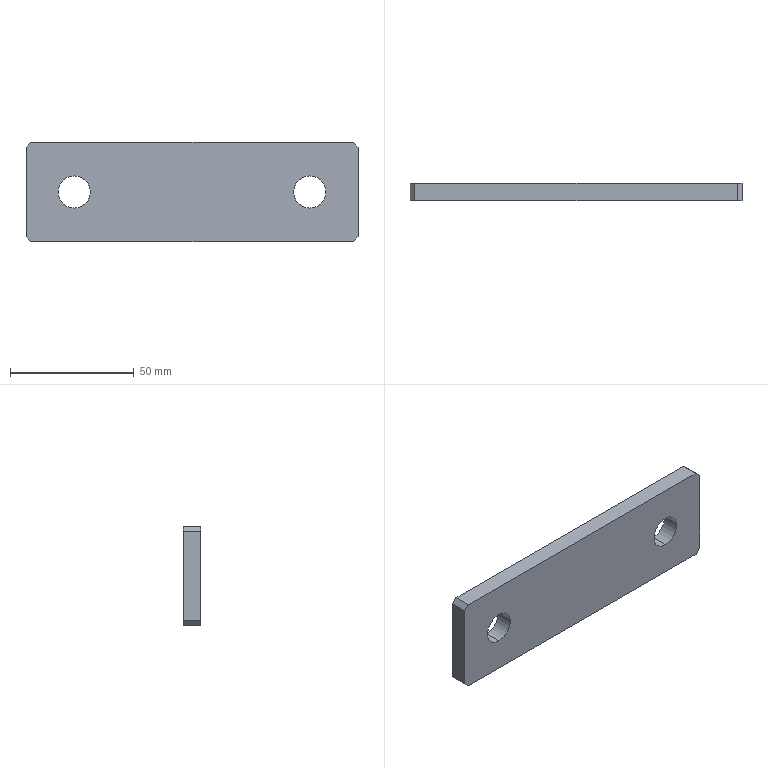Part | STEP file | 1004-2001-0021_1004-2001-0021_1-2 | 1 solid | 14 faces | box 134 x 7 x 40 mm | volume 35606 mm3 | plane 10 | cylinder 4 | commonest cylinder face diameters 13 x4
STEP:
#1=CARTESIAN_POINT('',(-47.5,-3.5,6.5));
#2=VERTEX_POINT('',#1);
#3=CARTESIAN_POINT('',(-47.5,-3.5,-6.5));
#4=VERTEX_POINT('',#3);
#5=CARTESIAN_POINT('',(-47.5,-3.5,0.));
#6=DIRECTION('',(0.,-1.,0.));
#7=DIRECTION('',(0.,0.,1.));
#8=AXIS2_PLACEMENT_3D('',#5,#6,#7);
#9=CIRCLE('',#8,6.5);
#10=EDGE_CURVE('',#2,#4,#9,.T.);
#11=ORIENTED_EDGE('',*,*,#10,.T.);
#12=CARTESIAN_POINT('',(-47.5,3.5,-6.5));
#13=VERTEX_POINT('',#12);
#14=CARTESIAN_POINT('',(-47.5,3.5,-6.5));
#15=DIRECTION('',(0.,1.,0.));
#16=VECTOR('',#15,1000.);
#17=LINE('',#14,#16);
#18=EDGE_CURVE('',#4,#13,#17,.T.);
#19=ORIENTED_EDGE('',*,*,#18,.T.);
#20=CARTESIAN_POINT('',(-47.5,3.5,6.5));
#21=VERTEX_POINT('',#20);
#22=CARTESIAN_POINT('',(-47.5,3.5,0.));
#23=DIRECTION('',(0.,-1.,0.));
#24=DIRECTION('',(0.,0.,1.));
#25=AXIS2_PLACEMENT_3D('',#22,#23,#24);
#26=CIRCLE('',#25,6.5);
#27=EDGE_CURVE('',#21,#13,#26,.T.);
#28=ORIENTED_EDGE('',*,*,#27,.F.);
#29=CARTESIAN_POINT('',(-47.5,3.5,6.5));
#30=DIRECTION('',(0.,1.,0.));
#31=VECTOR('',#30,1000.);
#32=LINE('',#29,#31);
#33=EDGE_CURVE('',#2,#21,#32,.T.);
#34=ORIENTED_EDGE('',*,*,#33,.F.);
#35=EDGE_LOOP('',(#11,#19,#28,#34));
#36=FACE_OUTER_BOUND('',#35,.T.);
#37=CARTESIAN_POINT('',(-47.5,3.5,0.));
#38=DIRECTION('',(0.,1.,0.));
#39=DIRECTION('',(0.,0.,1.));
#40=AXIS2_PLACEMENT_3D('',#37,#38,#39);
#41=CYLINDRICAL_SURFACE('',#40,6.5);
#42=ADVANCED_FACE('',(#36),#41,.F.);
#43=CARTESIAN_POINT('',(47.5,-3.5,6.5));
#44=VERTEX_POINT('',#43);
#45=CARTESIAN_POINT('',(47.5,-3.5,-6.5));
#46=VERTEX_POINT('',#45);
#47=CARTESIAN_POINT('',(47.5,-3.5,0.));
#48=DIRECTION('',(0.,-1.,0.));
#49=DIRECTION('',(0.,0.,1.));
#50=AXIS2_PLACEMENT_3D('',#47,#48,#49);
#51=CIRCLE('',#50,6.5);
#52=EDGE_CURVE('',#44,#46,#51,.T.);
#53=ORIENTED_EDGE('',*,*,#52,.T.);
#54=CARTESIAN_POINT('',(47.5,3.5,-6.5));
#55=VERTEX_POINT('',#54);
#56=CARTESIAN_POINT('',(47.5,3.5,-6.5));
#57=DIRECTION('',(0.,1.,0.));
#58=VECTOR('',#57,1000.);
#59=LINE('',#56,#58);
#60=EDGE_CURVE('',#46,#55,#59,.T.);
#61=ORIENTED_EDGE('',*,*,#60,.T.);
#62=CARTESIAN_POINT('',(47.5,3.5,6.5));
#63=VERTEX_POINT('',#62);
#64=CARTESIAN_POINT('',(47.5,3.5,0.));
#65=DIRECTION('',(0.,-1.,0.));
#66=DIRECTION('',(0.,0.,1.));
#67=AXIS2_PLACEMENT_3D('',#64,#65,#66);
#68=CIRCLE('',#67,6.5);
#69=EDGE_CURVE('',#63,#55,#68,.T.);
#70=ORIENTED_EDGE('',*,*,#69,.F.);
#71=CARTESIAN_POINT('',(47.5,3.5,6.5));
#72=DIRECTION('',(0.,1.,0.));
#73=VECTOR('',#72,1000.);
#74=LINE('',#71,#73);
#75=EDGE_CURVE('',#44,#63,#74,.T.);
#76=ORIENTED_EDGE('',*,*,#75,.F.);
#77=EDGE_LOOP('',(#53,#61,#70,#76));
#78=FACE_OUTER_BOUND('',#77,.T.);
#79=CARTESIAN_POINT('',(47.5,3.5,0.));
#80=DIRECTION('',(0.,1.,0.));
#81=DIRECTION('',(0.,0.,1.));
#82=AXIS2_PLACEMENT_3D('',#79,#80,#81);
#83=CYLINDRICAL_SURFACE('',#82,6.5);
#84=ADVANCED_FACE('',(#78),#83,.F.);
#85=ORIENTED_EDGE('',*,*,#10,.F.);
#86=CARTESIAN_POINT('',(-47.5,-3.5,0.));
#87=DIRECTION('',(0.,-1.,0.));
#88=DIRECTION('',(0.,0.,1.));
#89=AXIS2_PLACEMENT_3D('',#86,#87,#88);
#90=CIRCLE('',#89,6.5);
#91=EDGE_CURVE('',#4,#2,#90,.T.);
#92=ORIENTED_EDGE('',*,*,#91,.F.);
#93=EDGE_LOOP('',(#85,#92));
#94=FACE_BOUND('',#93,.T.);
#95=ORIENTED_EDGE('',*,*,#52,.F.);
#96=CARTESIAN_POINT('',(47.5,-3.5,0.));
#97=DIRECTION('',(0.,-1.,0.));
#98=DIRECTION('',(0.,0.,1.));
#99=AXIS2_PLACEMENT_3D('',#96,#97,#98);
#100=CIRCLE('',#99,6.5);
#101=EDGE_CURVE('',#46,#44,#100,.T.);
#102=ORIENTED_EDGE('',*,*,#101,.F.);
#103=EDGE_LOOP('',(#95,#102));
#104=FACE_BOUND('',#103,.T.);
#105=CARTESIAN_POINT('',(65.,-3.5,-20.));
#106=VERTEX_POINT('',#105);
#107=CARTESIAN_POINT('',(-65.,-3.5,-20.));
#108=VERTEX_POINT('',#107);
#109=CARTESIAN_POINT('',(67.,-3.5,-20.));
#110=DIRECTION('',(-1.,0.,0.));
#111=VECTOR('',#110,1000.);
#112=LINE('',#109,#111);
#113=EDGE_CURVE('',#106,#108,#112,.T.);
#114=ORIENTED_EDGE('',*,*,#113,.F.);
#115=CARTESIAN_POINT('',(67.,-3.5,-18.));
#116=VERTEX_POINT('',#115);
#117=CARTESIAN_POINT('',(67.,-3.5,-18.));
#118=DIRECTION('',(-0.7071,0.,-0.7071));
#119=VECTOR('',#118,1000.);
#120=LINE('',#117,#119);
#121=EDGE_CURVE('',#116,#106,#120,.T.);
#122=ORIENTED_EDGE('',*,*,#121,.F.);
#123=CARTESIAN_POINT('',(67.,-3.5,18.));
#124=VERTEX_POINT('',#123);
#125=CARTESIAN_POINT('',(67.,-3.5,-20.));
#126=DIRECTION('',(0.,0.,-1.));
#127=VECTOR('',#126,1000.);
#128=LINE('',#125,#127);
#129=EDGE_CURVE('',#124,#116,#128,.T.);
#130=ORIENTED_EDGE('',*,*,#129,.F.);
#131=CARTESIAN_POINT('',(65.,-3.5,20.));
#132=VERTEX_POINT('',#131);
#133=CARTESIAN_POINT('',(65.,-3.5,20.));
#134=DIRECTION('',(0.7071,0.,-0.7071));
#135=VECTOR('',#134,1000.);
#136=LINE('',#133,#135);
#137=EDGE_CURVE('',#132,#124,#136,.T.);
#138=ORIENTED_EDGE('',*,*,#137,.F.);
#139=CARTESIAN_POINT('',(-65.,-3.5,20.));
#140=VERTEX_POINT('',#139);
#141=CARTESIAN_POINT('',(67.,-3.5,20.));
#142=DIRECTION('',(1.,0.,0.));
#143=VECTOR('',#142,1000.);
#144=LINE('',#141,#143);
#145=EDGE_CURVE('',#140,#132,#144,.T.);
#146=ORIENTED_EDGE('',*,*,#145,.F.);
#147=CARTESIAN_POINT('',(-67.,-3.5,18.));
#148=VERTEX_POINT('',#147);
#149=CARTESIAN_POINT('',(-67.,-3.5,18.));
#150=DIRECTION('',(0.7071,0.,0.7071));
#151=VECTOR('',#150,1000.);
#152=LINE('',#149,#151);
#153=EDGE_CURVE('',#148,#140,#152,.T.);
#154=ORIENTED_EDGE('',*,*,#153,.F.);
#155=CARTESIAN_POINT('',(-67.,-3.5,-18.));
#156=VERTEX_POINT('',#155);
#157=CARTESIAN_POINT('',(-67.,-3.5,-20.));
#158=DIRECTION('',(0.,0.,1.));
#159=VECTOR('',#158,1000.);
#160=LINE('',#157,#159);
#161=EDGE_CURVE('',#156,#148,#160,.T.);
#162=ORIENTED_EDGE('',*,*,#161,.F.);
#163=CARTESIAN_POINT('',(-65.,-3.5,-20.));
#164=DIRECTION('',(-0.7071,0.,0.7071));
#165=VECTOR('',#164,1000.);
#166=LINE('',#163,#165);
#167=EDGE_CURVE('',#108,#156,#166,.T.);
#168=ORIENTED_EDGE('',*,*,#167,.F.);
#169=EDGE_LOOP('',(#114,#122,#130,#138,#146,#154,#162,#168));
#170=FACE_OUTER_BOUND('',#169,.T.);
#171=CARTESIAN_POINT('',(67.,-3.5,-20.));
#172=DIRECTION('',(0.,1.,0.));
#173=DIRECTION('',(0.,0.,1.));
#174=AXIS2_PLACEMENT_3D('',#171,#172,#173);
#175=PLANE('',#174);
#176=ADVANCED_FACE('',(#94,#104,#170),#175,.F.);
#177=ORIENTED_EDGE('',*,*,#18,.F.);
#178=ORIENTED_EDGE('',*,*,#91,.T.);
#179=ORIENTED_EDGE('',*,*,#33,.T.);
#180=CARTESIAN_POINT('',(-47.5,3.5,0.));
#181=DIRECTION('',(0.,-1.,0.));
#182=DIRECTION('',(0.,0.,1.));
#183=AXIS2_PLACEMENT_3D('',#180,#181,#182);
#184=CIRCLE('',#183,6.5);
#185=EDGE_CURVE('',#13,#21,#184,.T.);
#186=ORIENTED_EDGE('',*,*,#185,.F.);
#187=EDGE_LOOP('',(#177,#178,#179,#186));
#188=FACE_OUTER_BOUND('',#187,.T.);
#189=CARTESIAN_POINT('',(-47.5,3.5,0.));
#190=DIRECTION('',(0.,1.,0.));
#191=DIRECTION('',(0.,0.,1.));
#192=AXIS2_PLACEMENT_3D('',#189,#190,#191);
#193=CYLINDRICAL_SURFACE('',#192,6.5);
#194=ADVANCED_FACE('',(#188),#193,.F.);
#195=ORIENTED_EDGE('',*,*,#60,.F.);
#196=ORIENTED_EDGE('',*,*,#101,.T.);
#197=ORIENTED_EDGE('',*,*,#75,.T.);
#198=CARTESIAN_POINT('',(47.5,3.5,0.));
#199=DIRECTION('',(0.,-1.,0.));
#200=DIRECTION('',(0.,0.,1.));
#201=AXIS2_PLACEMENT_3D('',#198,#199,#200);
#202=CIRCLE('',#201,6.5);
#203=EDGE_CURVE('',#55,#63,#202,.T.);
#204=ORIENTED_EDGE('',*,*,#203,.F.);
#205=EDGE_LOOP('',(#195,#196,#197,#204));
#206=FACE_OUTER_BOUND('',#205,.T.);
#207=CARTESIAN_POINT('',(47.5,3.5,0.));
#208=DIRECTION('',(0.,1.,0.));
#209=DIRECTION('',(0.,0.,1.));
#210=AXIS2_PLACEMENT_3D('',#207,#208,#209);
#211=CYLINDRICAL_SURFACE('',#210,6.5);
#212=ADVANCED_FACE('',(#206),#211,.F.);
#213=CARTESIAN_POINT('',(-65.,3.5,-20.));
#214=VERTEX_POINT('',#213);
#215=CARTESIAN_POINT('',(-67.,3.5,-18.));
#216=VERTEX_POINT('',#215);
#217=CARTESIAN_POINT('',(-65.,3.5,-20.));
#218=DIRECTION('',(-0.7071,0.,0.7071));
#219=VECTOR('',#218,1000.);
#220=LINE('',#217,#219);
#221=EDGE_CURVE('',#214,#216,#220,.T.);
#222=ORIENTED_EDGE('',*,*,#221,.F.);
#223=CARTESIAN_POINT('',(-65.,-3.5,-20.));
#224=DIRECTION('',(0.,1.,0.));
#225=VECTOR('',#224,1000.);
#226=LINE('',#223,#225);
#227=EDGE_CURVE('',#108,#214,#226,.T.);
#228=ORIENTED_EDGE('',*,*,#227,.F.);
#229=ORIENTED_EDGE('',*,*,#167,.T.);
#230=CARTESIAN_POINT('',(-67.,-3.5,-18.));
#231=DIRECTION('',(0.,-1.,0.));
#232=VECTOR('',#231,1000.);
#233=LINE('',#230,#232);
#234=EDGE_CURVE('',#216,#156,#233,.T.);
#235=ORIENTED_EDGE('',*,*,#234,.F.);
#236=EDGE_LOOP('',(#222,#228,#229,#235));
#237=FACE_OUTER_BOUND('',#236,.T.);
#238=CARTESIAN_POINT('',(-65.,-3.5,-20.));
#239=DIRECTION('',(0.7071,0.,0.7071));
#240=DIRECTION('',(0.7071,0.,-0.7071));
#241=AXIS2_PLACEMENT_3D('',#238,#239,#240);
#242=PLANE('',#241);
#243=ADVANCED_FACE('',(#237),#242,.F.);
#244=CARTESIAN_POINT('',(65.,3.5,-20.));
#245=VERTEX_POINT('',#244);
#246=CARTESIAN_POINT('',(67.,3.5,-20.));
#247=DIRECTION('',(-1.,0.,0.));
#248=VECTOR('',#247,1000.);
#249=LINE('',#246,#248);
#250=EDGE_CURVE('',#245,#214,#249,.T.);
#251=ORIENTED_EDGE('',*,*,#250,.F.);
#252=CARTESIAN_POINT('',(65.,-3.5,-20.));
#253=DIRECTION('',(0.,1.,0.));
#254=VECTOR('',#253,1000.);
#255=LINE('',#252,#254);
#256=EDGE_CURVE('',#106,#245,#255,.T.);
#257=ORIENTED_EDGE('',*,*,#256,.F.);
#258=ORIENTED_EDGE('',*,*,#113,.T.);
#259=ORIENTED_EDGE('',*,*,#227,.T.);
#260=EDGE_LOOP('',(#251,#257,#258,#259));
#261=FACE_OUTER_BOUND('',#260,.T.);
#262=CARTESIAN_POINT('',(67.,-3.5,-20.));
#263=DIRECTION('',(0.,0.,1.));
#264=DIRECTION('',(1.,0.,0.));
#265=AXIS2_PLACEMENT_3D('',#262,#263,#264);
#266=PLANE('',#265);
#267=ADVANCED_FACE('',(#261),#266,.F.);
#268=CARTESIAN_POINT('',(67.,3.5,-18.));
#269=VERTEX_POINT('',#268);
#270=CARTESIAN_POINT('',(67.,3.5,-18.));
#271=DIRECTION('',(0.,-1.,0.));
#272=VECTOR('',#271,1000.);
#273=LINE('',#270,#272);
#274=EDGE_CURVE('',#269,#116,#273,.T.);
#275=ORIENTED_EDGE('',*,*,#274,.T.);
#276=ORIENTED_EDGE('',*,*,#121,.T.);
#277=ORIENTED_EDGE('',*,*,#256,.T.);
#278=CARTESIAN_POINT('',(67.,3.5,-18.));
#279=DIRECTION('',(0.7071,0.,0.7071));
#280=VECTOR('',#279,1000.);
#281=LINE('',#278,#280);
#282=EDGE_CURVE('',#245,#269,#281,.T.);
#283=ORIENTED_EDGE('',*,*,#282,.T.);
#284=EDGE_LOOP('',(#275,#276,#277,#283));
#285=FACE_OUTER_BOUND('',#284,.T.);
#286=CARTESIAN_POINT('',(67.,3.5,-18.));
#287=DIRECTION('',(0.7071,0.,-0.7071));
#288=DIRECTION('',(-0.7071,0.,-0.7071));
#289=AXIS2_PLACEMENT_3D('',#286,#287,#288);
#290=PLANE('',#289);
#291=ADVANCED_FACE('',(#285),#290,.T.);
#292=CARTESIAN_POINT('',(67.,3.5,18.));
#293=VERTEX_POINT('',#292);
#294=CARTESIAN_POINT('',(67.,3.5,18.));
#295=DIRECTION('',(0.,-1.,0.));
#296=VECTOR('',#295,1000.);
#297=LINE('',#294,#296);
#298=EDGE_CURVE('',#293,#124,#297,.T.);
#299=ORIENTED_EDGE('',*,*,#298,.T.);
#300=ORIENTED_EDGE('',*,*,#129,.T.);
#301=ORIENTED_EDGE('',*,*,#274,.F.);
#302=CARTESIAN_POINT('',(67.,3.5,20.));
#303=DIRECTION('',(0.,0.,1.));
#304=VECTOR('',#303,1000.);
#305=LINE('',#302,#304);
#306=EDGE_CURVE('',#269,#293,#305,.T.);
#307=ORIENTED_EDGE('',*,*,#306,.T.);
#308=EDGE_LOOP('',(#299,#300,#301,#307));
#309=FACE_OUTER_BOUND('',#308,.T.);
#310=CARTESIAN_POINT('',(67.,3.5,20.));
#311=DIRECTION('',(1.,0.,0.));
#312=DIRECTION('',(0.,0.,-1.));
#313=AXIS2_PLACEMENT_3D('',#310,#311,#312);
#314=PLANE('',#313);
#315=ADVANCED_FACE('',(#309),#314,.T.);
#316=ORIENTED_EDGE('',*,*,#298,.F.);
#317=CARTESIAN_POINT('',(65.,3.5,20.));
#318=VERTEX_POINT('',#317);
#319=CARTESIAN_POINT('',(67.,3.5,18.));
#320=DIRECTION('',(-0.7071,0.,0.7071));
#321=VECTOR('',#320,1000.);
#322=LINE('',#319,#321);
#323=EDGE_CURVE('',#293,#318,#322,.T.);
#324=ORIENTED_EDGE('',*,*,#323,.T.);
#325=CARTESIAN_POINT('',(65.,3.5,20.));
#326=DIRECTION('',(0.,-1.,0.));
#327=VECTOR('',#326,1000.);
#328=LINE('',#325,#327);
#329=EDGE_CURVE('',#318,#132,#328,.T.);
#330=ORIENTED_EDGE('',*,*,#329,.T.);
#331=ORIENTED_EDGE('',*,*,#137,.T.);
#332=EDGE_LOOP('',(#316,#324,#330,#331));
#333=FACE_OUTER_BOUND('',#332,.T.);
#334=CARTESIAN_POINT('',(67.,3.5,18.));
#335=DIRECTION('',(0.7071,0.,0.7071));
#336=DIRECTION('',(0.7071,0.,-0.7071));
#337=AXIS2_PLACEMENT_3D('',#334,#335,#336);
#338=PLANE('',#337);
#339=ADVANCED_FACE('',(#333),#338,.T.);
#340=CARTESIAN_POINT('',(-65.,3.5,20.));
#341=VERTEX_POINT('',#340);
#342=CARTESIAN_POINT('',(67.,3.5,20.));
#343=DIRECTION('',(1.,0.,0.));
#344=VECTOR('',#343,1000.);
#345=LINE('',#342,#344);
#346=EDGE_CURVE('',#341,#318,#345,.T.);
#347=ORIENTED_EDGE('',*,*,#346,.F.);
#348=CARTESIAN_POINT('',(-65.,-3.5,20.));
#349=DIRECTION('',(0.,1.,0.));
#350=VECTOR('',#349,1000.);
#351=LINE('',#348,#350);
#352=EDGE_CURVE('',#140,#341,#351,.T.);
#353=ORIENTED_EDGE('',*,*,#352,.F.);
#354=ORIENTED_EDGE('',*,*,#145,.T.);
#355=ORIENTED_EDGE('',*,*,#329,.F.);
#356=EDGE_LOOP('',(#347,#353,#354,#355));
#357=FACE_OUTER_BOUND('',#356,.T.);
#358=CARTESIAN_POINT('',(67.,-3.5,20.));
#359=DIRECTION('',(0.,0.,-1.));
#360=DIRECTION('',(-1.,0.,0.));
#361=AXIS2_PLACEMENT_3D('',#358,#359,#360);
#362=PLANE('',#361);
#363=ADVANCED_FACE('',(#357),#362,.F.);
#364=ORIENTED_EDGE('',*,*,#153,.T.);
#365=ORIENTED_EDGE('',*,*,#352,.T.);
#366=CARTESIAN_POINT('',(-67.,3.5,18.));
#367=VERTEX_POINT('',#366);
#368=CARTESIAN_POINT('',(-65.,3.5,20.));
#369=DIRECTION('',(0.7071,0.,0.7071));
#370=VECTOR('',#369,1000.);
#371=LINE('',#368,#370);
#372=EDGE_CURVE('',#367,#341,#371,.T.);
#373=ORIENTED_EDGE('',*,*,#372,.F.);
#374=CARTESIAN_POINT('',(-67.,-3.5,18.));
#375=DIRECTION('',(0.,1.,0.));
#376=VECTOR('',#375,1000.);
#377=LINE('',#374,#376);
#378=EDGE_CURVE('',#148,#367,#377,.T.);
#379=ORIENTED_EDGE('',*,*,#378,.F.);
#380=EDGE_LOOP('',(#364,#365,#373,#379));
#381=FACE_OUTER_BOUND('',#380,.T.);
#382=CARTESIAN_POINT('',(-65.,-3.5,20.));
#383=DIRECTION('',(0.7071,0.,-0.7071));
#384=DIRECTION('',(-0.7071,0.,-0.7071));
#385=AXIS2_PLACEMENT_3D('',#382,#383,#384);
#386=PLANE('',#385);
#387=ADVANCED_FACE('',(#381),#386,.F.);
#388=ORIENTED_EDGE('',*,*,#161,.T.);
#389=ORIENTED_EDGE('',*,*,#378,.T.);
#390=CARTESIAN_POINT('',(-67.,3.5,20.));
#391=DIRECTION('',(0.,0.,1.));
#392=VECTOR('',#391,1000.);
#393=LINE('',#390,#392);
#394=EDGE_CURVE('',#216,#367,#393,.T.);
#395=ORIENTED_EDGE('',*,*,#394,.F.);
#396=ORIENTED_EDGE('',*,*,#234,.T.);
#397=EDGE_LOOP('',(#388,#389,#395,#396));
#398=FACE_OUTER_BOUND('',#397,.T.);
#399=CARTESIAN_POINT('',(-67.,3.5,20.));
#400=DIRECTION('',(1.,0.,0.));
#401=DIRECTION('',(0.,0.,-1.));
#402=AXIS2_PLACEMENT_3D('',#399,#400,#401);
#403=PLANE('',#402);
#404=ADVANCED_FACE('',(#398),#403,.F.);
#405=ORIENTED_EDGE('',*,*,#27,.T.);
#406=ORIENTED_EDGE('',*,*,#185,.T.);
#407=EDGE_LOOP('',(#405,#406));
#408=FACE_BOUND('',#407,.T.);
#409=ORIENTED_EDGE('',*,*,#69,.T.);
#410=ORIENTED_EDGE('',*,*,#203,.T.);
#411=EDGE_LOOP('',(#409,#410));
#412=FACE_BOUND('',#411,.T.);
#413=ORIENTED_EDGE('',*,*,#394,.T.);
#414=ORIENTED_EDGE('',*,*,#372,.T.);
#415=ORIENTED_EDGE('',*,*,#346,.T.);
#416=ORIENTED_EDGE('',*,*,#323,.F.);
#417=ORIENTED_EDGE('',*,*,#306,.F.);
#418=ORIENTED_EDGE('',*,*,#282,.F.);
#419=ORIENTED_EDGE('',*,*,#250,.T.);
#420=ORIENTED_EDGE('',*,*,#221,.T.);
#421=EDGE_LOOP('',(#413,#414,#415,#416,#417,#418,#419,#420));
#422=FACE_OUTER_BOUND('',#421,.T.);
#423=CARTESIAN_POINT('',(67.,3.5,-20.));
#424=DIRECTION('',(0.,-1.,0.));
#425=DIRECTION('',(0.,0.,-1.));
#426=AXIS2_PLACEMENT_3D('',#423,#424,#425);
#427=PLANE('',#426);
#428=ADVANCED_FACE('',(#408,#412,#422),#427,.F.);
#429=CLOSED_SHELL('',(#42,#84,#176,#194,#212,#243,#267,#291,#315,#339,#363,#387,#404,#428));
#430=MANIFOLD_SOLID_BREP('',#429);
#431=CARTESIAN_POINT('',(0.,0.,0.));
#432=DIRECTION('',(0.,0.,1.));
#433=DIRECTION('',(1.,0.,0.));
#434=AXIS2_PLACEMENT_3D('',#431,#432,#433);
#435=(LENGTH_UNIT()NAMED_UNIT(*)SI_UNIT(.MILLI.,.METRE.));
#436=UNCERTAINTY_MEASURE_WITH_UNIT(LENGTH_MEASURE(0.00001),#435,'','');
#437=(NAMED_UNIT(*)PLANE_ANGLE_UNIT()SI_UNIT($,.RADIAN.));
#438=(NAMED_UNIT(*)SI_UNIT($,.STERADIAN.)SOLID_ANGLE_UNIT());
#439=(GEOMETRIC_REPRESENTATION_CONTEXT(3)GLOBAL_UNCERTAINTY_ASSIGNED_CONTEXT((#436))GLOBAL_UNIT_ASSIGNED_CONTEXT((#435,#437,#438))REPRESENTATION_CONTEXT('',''));
#440=ADVANCED_BREP_SHAPE_REPRESENTATION('',(#430,#434),#439);